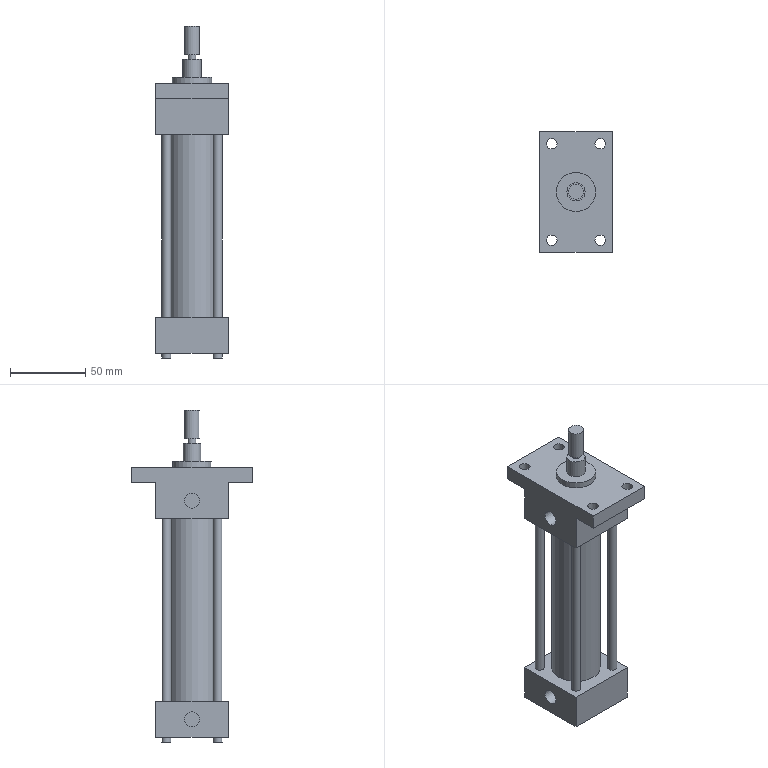Part | NX | features solid 2 | 1 solid | 48 faces | box 48 x 80 x 220 mm | volume 193287 mm3 | plane 28 | cylinder 20 | commonest cylinder face diameters 6 x8 7 x4 10 x3 5 x1 12 x1 26 x1
STEP:
#1=CARTESIAN_POINT('',(-500.,9.,-224.));
#2=VERTEX_POINT('',#1);
#3=CARTESIAN_POINT('',(-516.,9.,-224.));
#4=DIRECTION('',(0.,0.,-1.));
#5=DIRECTION('',(1.,0.,0.));
#6=AXIS2_PLACEMENT_3D('',#3,#4,#5);
#7=CIRCLE('',#6,16.);
#8=EDGE_CURVE('',#2,#2,#7,.T.);
#9=ORIENTED_EDGE('',*,*,#8,.T.);
#10=EDGE_LOOP('',(#9));
#11=FACE_BOUND('',#10,.T.);
#12=CARTESIAN_POINT('',(-500.,9.,-345.));
#13=VERTEX_POINT('',#12);
#14=CARTESIAN_POINT('',(-516.,9.,-345.));
#15=DIRECTION('',(0.,0.,-1.));
#16=DIRECTION('',(1.,0.,0.));
#17=AXIS2_PLACEMENT_3D('',#14,#15,#16);
#18=CIRCLE('',#17,16.);
#19=EDGE_CURVE('',#13,#13,#18,.F.);
#20=ORIENTED_EDGE('',*,*,#19,.T.);
#21=EDGE_LOOP('',(#20));
#22=FACE_BOUND('',#21,.T.);
#23=CARTESIAN_POINT('',(-516.,9.,-369.));
#24=DIRECTION('',(0.,0.,1.));
#25=DIRECTION('',(-1.,0.,0.));
#26=AXIS2_PLACEMENT_3D('',#23,#24,#25);
#27=CYLINDRICAL_SURFACE('',#26,16.);
#28=ADVANCED_FACE('',(#11,#22),#27,.T.);
#29=CARTESIAN_POINT('',(-522.,9.,-174.));
#30=VERTEX_POINT('',#29);
#31=CARTESIAN_POINT('',(-516.,9.,-174.));
#32=DIRECTION('',(0.,0.,1.));
#33=DIRECTION('',(-1.,0.,0.));
#34=AXIS2_PLACEMENT_3D('',#31,#32,#33);
#35=CIRCLE('',#34,6.);
#36=EDGE_CURVE('',#30,#30,#35,.T.);
#37=ORIENTED_EDGE('',*,*,#36,.T.);
#38=EDGE_LOOP('',(#37));
#39=FACE_BOUND('',#38,.T.);
#40=CARTESIAN_POINT('',(-518.5,9.,-174.));
#41=VERTEX_POINT('',#40);
#42=CARTESIAN_POINT('',(-516.,9.,-174.));
#43=DIRECTION('',(0.,0.,1.));
#44=DIRECTION('',(-1.,0.,0.));
#45=AXIS2_PLACEMENT_3D('',#42,#43,#44);
#46=CIRCLE('',#45,2.5);
#47=EDGE_CURVE('',#41,#41,#46,.T.);
#48=ORIENTED_EDGE('',*,*,#47,.F.);
#49=EDGE_LOOP('',(#48));
#50=FACE_BOUND('',#49,.T.);
#51=CARTESIAN_POINT('',(-516.,9.,-174.));
#52=DIRECTION('',(0.,0.,1.));
#53=DIRECTION('',(-1.,0.,0.));
#54=AXIS2_PLACEMENT_3D('',#51,#52,#53);
#55=PLANE('',#54);
#56=ADVANCED_FACE('',(#39,#50),#55,.T.);
#57=CARTESIAN_POINT('',(-529.,9.,-186.));
#58=VERTEX_POINT('',#57);
#59=CARTESIAN_POINT('',(-516.,9.,-186.));
#60=DIRECTION('',(0.,0.,1.));
#61=DIRECTION('',(-1.,0.,0.));
#62=AXIS2_PLACEMENT_3D('',#59,#60,#61);
#63=CIRCLE('',#62,13.);
#64=EDGE_CURVE('',#58,#58,#63,.T.);
#65=ORIENTED_EDGE('',*,*,#64,.T.);
#66=EDGE_LOOP('',(#65));
#67=FACE_BOUND('',#66,.T.);
#68=CARTESIAN_POINT('',(-522.,9.,-186.));
#69=VERTEX_POINT('',#68);
#70=CARTESIAN_POINT('',(-516.,9.,-186.));
#71=DIRECTION('',(0.,0.,1.));
#72=DIRECTION('',(-1.,0.,0.));
#73=AXIS2_PLACEMENT_3D('',#70,#71,#72);
#74=CIRCLE('',#73,6.);
#75=EDGE_CURVE('',#69,#69,#74,.F.);
#76=ORIENTED_EDGE('',*,*,#75,.T.);
#77=EDGE_LOOP('',(#76));
#78=FACE_BOUND('',#77,.T.);
#79=CARTESIAN_POINT('',(-516.,9.,-186.));
#80=DIRECTION('',(0.,0.,1.));
#81=DIRECTION('',(-1.,0.,0.));
#82=AXIS2_PLACEMENT_3D('',#79,#80,#81);
#83=PLANE('',#82);
#84=ADVANCED_FACE('',(#67,#78),#83,.T.);
#85=CARTESIAN_POINT('',(-503.5,41.,-190.));
#86=VERTEX_POINT('',#85);
#87=CARTESIAN_POINT('',(-500.,41.,-190.));
#88=DIRECTION('',(0.,0.,1.));
#89=DIRECTION('',(-1.,0.,0.));
#90=AXIS2_PLACEMENT_3D('',#87,#88,#89);
#91=CIRCLE('',#90,3.5);
#92=EDGE_CURVE('',#86,#86,#91,.T.);
#93=ORIENTED_EDGE('',*,*,#92,.F.);
#94=EDGE_LOOP('',(#93));
#95=FACE_BOUND('',#94,.T.);
#96=CARTESIAN_POINT('',(-535.5,-23.,-190.));
#97=VERTEX_POINT('',#96);
#98=CARTESIAN_POINT('',(-532.,-23.,-190.));
#99=DIRECTION('',(0.,0.,1.));
#100=DIRECTION('',(-1.,0.,0.));
#101=AXIS2_PLACEMENT_3D('',#98,#99,#100);
#102=CIRCLE('',#101,3.5);
#103=EDGE_CURVE('',#97,#97,#102,.T.);
#104=ORIENTED_EDGE('',*,*,#103,.F.);
#105=EDGE_LOOP('',(#104));
#106=FACE_BOUND('',#105,.T.);
#107=CARTESIAN_POINT('',(-492.,-31.,-190.));
#108=VERTEX_POINT('',#107);
#109=CARTESIAN_POINT('',(-540.,-31.,-190.));
#110=VERTEX_POINT('',#109);
#111=CARTESIAN_POINT('',(-492.,-31.,-190.));
#112=DIRECTION('',(-1.,0.,0.));
#113=VECTOR('',#112,1000.);
#114=LINE('',#111,#113);
#115=EDGE_CURVE('',#108,#110,#114,.T.);
#116=ORIENTED_EDGE('',*,*,#115,.F.);
#117=CARTESIAN_POINT('',(-492.,49.,-190.));
#118=VERTEX_POINT('',#117);
#119=CARTESIAN_POINT('',(-492.,-15.,-190.));
#120=DIRECTION('',(0.,-1.,0.));
#121=VECTOR('',#120,1000.);
#122=LINE('',#119,#121);
#123=EDGE_CURVE('',#118,#108,#122,.T.);
#124=ORIENTED_EDGE('',*,*,#123,.F.);
#125=CARTESIAN_POINT('',(-540.,49.,-190.));
#126=VERTEX_POINT('',#125);
#127=CARTESIAN_POINT('',(-492.,49.,-190.));
#128=DIRECTION('',(-1.,0.,0.));
#129=VECTOR('',#128,1000.);
#130=LINE('',#127,#129);
#131=EDGE_CURVE('',#118,#126,#130,.T.);
#132=ORIENTED_EDGE('',*,*,#131,.T.);
#133=CARTESIAN_POINT('',(-540.,49.,-190.));
#134=DIRECTION('',(0.,-1.,0.));
#135=VECTOR('',#134,1000.);
#136=LINE('',#133,#135);
#137=EDGE_CURVE('',#126,#110,#136,.T.);
#138=ORIENTED_EDGE('',*,*,#137,.T.);
#139=EDGE_LOOP('',(#116,#124,#132,#138));
#140=FACE_BOUND('',#139,.T.);
#141=CARTESIAN_POINT('',(-503.5,-23.,-190.));
#142=VERTEX_POINT('',#141);
#143=CARTESIAN_POINT('',(-500.,-23.,-190.));
#144=DIRECTION('',(0.,0.,1.));
#145=DIRECTION('',(-1.,0.,0.));
#146=AXIS2_PLACEMENT_3D('',#143,#144,#145);
#147=CIRCLE('',#146,3.5);
#148=EDGE_CURVE('',#142,#142,#147,.T.);
#149=ORIENTED_EDGE('',*,*,#148,.F.);
#150=EDGE_LOOP('',(#149));
#151=FACE_BOUND('',#150,.T.);
#152=CARTESIAN_POINT('',(-535.5,41.,-190.));
#153=VERTEX_POINT('',#152);
#154=CARTESIAN_POINT('',(-532.,41.,-190.));
#155=DIRECTION('',(0.,0.,1.));
#156=DIRECTION('',(-1.,0.,0.));
#157=AXIS2_PLACEMENT_3D('',#154,#155,#156);
#158=CIRCLE('',#157,3.5);
#159=EDGE_CURVE('',#153,#153,#158,.T.);
#160=ORIENTED_EDGE('',*,*,#159,.F.);
#161=EDGE_LOOP('',(#160));
#162=FACE_BOUND('',#161,.T.);
#163=CARTESIAN_POINT('',(-503.,9.,-190.));
#164=VERTEX_POINT('',#163);
#165=CARTESIAN_POINT('',(-516.,9.,-190.));
#166=DIRECTION('',(0.,0.,-1.));
#167=DIRECTION('',(1.,0.,0.));
#168=AXIS2_PLACEMENT_3D('',#165,#166,#167);
#169=CIRCLE('',#168,13.);
#170=EDGE_CURVE('',#164,#164,#169,.F.);
#171=ORIENTED_EDGE('',*,*,#170,.F.);
#172=EDGE_LOOP('',(#171));
#173=FACE_BOUND('',#172,.T.);
#174=CARTESIAN_POINT('',(-540.,-31.,-190.));
#175=DIRECTION('',(0.,0.,-1.));
#176=DIRECTION('',(1.,0.,0.));
#177=AXIS2_PLACEMENT_3D('',#174,#175,#176);
#178=PLANE('',#177);
#179=ADVANCED_FACE('',(#95,#106,#140,#151,#162,#173),#178,.F.);
#180=CARTESIAN_POINT('',(-540.,33.,-200.));
#181=VERTEX_POINT('',#180);
#182=CARTESIAN_POINT('',(-492.,33.,-200.));
#183=VERTEX_POINT('',#182);
#184=CARTESIAN_POINT('',(-540.,33.,-200.));
#185=DIRECTION('',(1.,0.,0.));
#186=VECTOR('',#185,1000.);
#187=LINE('',#184,#186);
#188=EDGE_CURVE('',#181,#183,#187,.T.);
#189=ORIENTED_EDGE('',*,*,#188,.F.);
#190=CARTESIAN_POINT('',(-540.,49.,-200.));
#191=VERTEX_POINT('',#190);
#192=CARTESIAN_POINT('',(-540.,49.,-200.));
#193=DIRECTION('',(0.,-1.,0.));
#194=VECTOR('',#193,1000.);
#195=LINE('',#192,#194);
#196=EDGE_CURVE('',#191,#181,#195,.T.);
#197=ORIENTED_EDGE('',*,*,#196,.F.);
#198=CARTESIAN_POINT('',(-492.,49.,-200.));
#199=VERTEX_POINT('',#198);
#200=CARTESIAN_POINT('',(-492.,49.,-200.));
#201=DIRECTION('',(-1.,0.,0.));
#202=VECTOR('',#201,1000.);
#203=LINE('',#200,#202);
#204=EDGE_CURVE('',#199,#191,#203,.T.);
#205=ORIENTED_EDGE('',*,*,#204,.F.);
#206=CARTESIAN_POINT('',(-492.,-15.,-200.));
#207=DIRECTION('',(0.,-1.,0.));
#208=VECTOR('',#207,1000.);
#209=LINE('',#206,#208);
#210=EDGE_CURVE('',#199,#183,#209,.T.);
#211=ORIENTED_EDGE('',*,*,#210,.T.);
#212=EDGE_LOOP('',(#189,#197,#205,#211));
#213=FACE_BOUND('',#212,.T.);
#214=CARTESIAN_POINT('',(-503.5,41.,-200.));
#215=VERTEX_POINT('',#214);
#216=CARTESIAN_POINT('',(-500.,41.,-200.));
#217=DIRECTION('',(0.,0.,1.));
#218=DIRECTION('',(-1.,0.,0.));
#219=AXIS2_PLACEMENT_3D('',#216,#217,#218);
#220=CIRCLE('',#219,3.5);
#221=EDGE_CURVE('',#215,#215,#220,.T.);
#222=ORIENTED_EDGE('',*,*,#221,.T.);
#223=EDGE_LOOP('',(#222));
#224=FACE_BOUND('',#223,.T.);
#225=CARTESIAN_POINT('',(-535.5,41.,-200.));
#226=VERTEX_POINT('',#225);
#227=CARTESIAN_POINT('',(-532.,41.,-200.));
#228=DIRECTION('',(0.,0.,1.));
#229=DIRECTION('',(-1.,0.,0.));
#230=AXIS2_PLACEMENT_3D('',#227,#228,#229);
#231=CIRCLE('',#230,3.5);
#232=EDGE_CURVE('',#226,#226,#231,.T.);
#233=ORIENTED_EDGE('',*,*,#232,.T.);
#234=EDGE_LOOP('',(#233));
#235=FACE_BOUND('',#234,.T.);
#236=CARTESIAN_POINT('',(-540.,-31.,-200.));
#237=DIRECTION('',(0.,0.,-1.));
#238=DIRECTION('',(1.,0.,0.));
#239=AXIS2_PLACEMENT_3D('',#236,#237,#238);
#240=PLANE('',#239);
#241=ADVANCED_FACE('',(#213,#224,#235),#240,.T.);
#242=ORIENTED_EDGE('',*,*,#115,.T.);
#243=CARTESIAN_POINT('',(-540.,-31.,-200.));
#244=VERTEX_POINT('',#243);
#245=CARTESIAN_POINT('',(-540.,-31.,-200.));
#246=DIRECTION('',(0.,0.,1.));
#247=VECTOR('',#246,1000.);
#248=LINE('',#245,#247);
#249=EDGE_CURVE('',#244,#110,#248,.T.);
#250=ORIENTED_EDGE('',*,*,#249,.F.);
#251=CARTESIAN_POINT('',(-492.,-31.,-200.));
#252=VERTEX_POINT('',#251);
#253=CARTESIAN_POINT('',(-492.,-31.,-200.));
#254=DIRECTION('',(-1.,0.,0.));
#255=VECTOR('',#254,1000.);
#256=LINE('',#253,#255);
#257=EDGE_CURVE('',#252,#244,#256,.T.);
#258=ORIENTED_EDGE('',*,*,#257,.F.);
#259=CARTESIAN_POINT('',(-492.,-31.,-200.));
#260=DIRECTION('',(0.,0.,1.));
#261=VECTOR('',#260,1000.);
#262=LINE('',#259,#261);
#263=EDGE_CURVE('',#252,#108,#262,.T.);
#264=ORIENTED_EDGE('',*,*,#263,.T.);
#265=EDGE_LOOP('',(#242,#250,#258,#264));
#266=FACE_BOUND('',#265,.T.);
#267=CARTESIAN_POINT('',(-492.,-31.,-200.));
#268=DIRECTION('',(0.,1.,0.));
#269=DIRECTION('',(0.,0.,-1.));
#270=AXIS2_PLACEMENT_3D('',#267,#268,#269);
#271=PLANE('',#270);
#272=ADVANCED_FACE('',(#266),#271,.F.);
#273=CARTESIAN_POINT('',(-540.,14.,-212.));
#274=VERTEX_POINT('',#273);
#275=CARTESIAN_POINT('',(-540.,9.,-212.));
#276=DIRECTION('',(1.,0.,0.));
#277=DIRECTION('',(0.,1.,0.));
#278=AXIS2_PLACEMENT_3D('',#275,#276,#277);
#279=CIRCLE('',#278,5.);
#280=EDGE_CURVE('',#274,#274,#279,.T.);
#281=ORIENTED_EDGE('',*,*,#280,.T.);
#282=EDGE_LOOP('',(#281));
#283=FACE_BOUND('',#282,.T.);
#284=ORIENTED_EDGE('',*,*,#137,.F.);
#285=CARTESIAN_POINT('',(-540.,49.,-200.));
#286=DIRECTION('',(0.,0.,1.));
#287=VECTOR('',#286,1000.);
#288=LINE('',#285,#287);
#289=EDGE_CURVE('',#191,#126,#288,.T.);
#290=ORIENTED_EDGE('',*,*,#289,.F.);
#291=ORIENTED_EDGE('',*,*,#196,.T.);
#292=CARTESIAN_POINT('',(-540.,33.,-224.));
#293=VERTEX_POINT('',#292);
#294=CARTESIAN_POINT('',(-540.,33.,-224.));
#295=DIRECTION('',(0.,0.,1.));
#296=VECTOR('',#295,1000.);
#297=LINE('',#294,#296);
#298=EDGE_CURVE('',#293,#181,#297,.T.);
#299=ORIENTED_EDGE('',*,*,#298,.F.);
#300=CARTESIAN_POINT('',(-540.,-15.,-224.));
#301=VERTEX_POINT('',#300);
#302=CARTESIAN_POINT('',(-540.,-15.,-224.));
#303=DIRECTION('',(0.,1.,0.));
#304=VECTOR('',#303,1000.);
#305=LINE('',#302,#304);
#306=EDGE_CURVE('',#301,#293,#305,.T.);
#307=ORIENTED_EDGE('',*,*,#306,.F.);
#308=CARTESIAN_POINT('',(-540.,-15.,-200.));
#309=VERTEX_POINT('',#308);
#310=CARTESIAN_POINT('',(-540.,-15.,-224.));
#311=DIRECTION('',(0.,0.,1.));
#312=VECTOR('',#311,1000.);
#313=LINE('',#310,#312);
#314=EDGE_CURVE('',#301,#309,#313,.T.);
#315=ORIENTED_EDGE('',*,*,#314,.T.);
#316=CARTESIAN_POINT('',(-540.,49.,-200.));
#317=DIRECTION('',(0.,-1.,0.));
#318=VECTOR('',#317,1000.);
#319=LINE('',#316,#318);
#320=EDGE_CURVE('',#309,#244,#319,.T.);
#321=ORIENTED_EDGE('',*,*,#320,.T.);
#322=ORIENTED_EDGE('',*,*,#249,.T.);
#323=EDGE_LOOP('',(#284,#290,#291,#299,#307,#315,#321,#322));
#324=FACE_BOUND('',#323,.T.);
#325=CARTESIAN_POINT('',(-540.,49.,-200.));
#326=DIRECTION('',(-1.,0.,0.));
#327=DIRECTION('',(0.,-1.,0.));
#328=AXIS2_PLACEMENT_3D('',#325,#326,#327);
#329=PLANE('',#328);
#330=ADVANCED_FACE('',(#283,#324),#329,.T.);
#331=ORIENTED_EDGE('',*,*,#131,.F.);
#332=CARTESIAN_POINT('',(-492.,49.,-200.));
#333=DIRECTION('',(0.,0.,1.));
#334=VECTOR('',#333,1000.);
#335=LINE('',#332,#334);
#336=EDGE_CURVE('',#199,#118,#335,.T.);
#337=ORIENTED_EDGE('',*,*,#336,.F.);
#338=ORIENTED_EDGE('',*,*,#204,.T.);
#339=ORIENTED_EDGE('',*,*,#289,.T.);
#340=EDGE_LOOP('',(#331,#337,#338,#339));
#341=FACE_BOUND('',#340,.T.);
#342=CARTESIAN_POINT('',(-492.,49.,-200.));
#343=DIRECTION('',(0.,1.,0.));
#344=DIRECTION('',(0.,0.,-1.));
#345=AXIS2_PLACEMENT_3D('',#342,#343,#344);
#346=PLANE('',#345);
#347=ADVANCED_FACE('',(#341),#346,.T.);
#348=CARTESIAN_POINT('',(-535.5,-23.,-200.));
#349=VERTEX_POINT('',#348);
#350=CARTESIAN_POINT('',(-532.,-23.,-200.));
#351=DIRECTION('',(0.,0.,1.));
#352=DIRECTION('',(-1.,0.,0.));
#353=AXIS2_PLACEMENT_3D('',#350,#351,#352);
#354=CIRCLE('',#353,3.5);
#355=EDGE_CURVE('',#349,#349,#354,.T.);
#356=ORIENTED_EDGE('',*,*,#355,.F.);
#357=EDGE_LOOP('',(#356));
#358=FACE_BOUND('',#357,.T.);
#359=ORIENTED_EDGE('',*,*,#103,.T.);
#360=EDGE_LOOP('',(#359));
#361=FACE_BOUND('',#360,.T.);
#362=CARTESIAN_POINT('',(-532.,-23.,-200.));
#363=DIRECTION('',(0.,0.,1.));
#364=DIRECTION('',(-1.,0.,0.));
#365=AXIS2_PLACEMENT_3D('',#362,#363,#364);
#366=CYLINDRICAL_SURFACE('',#365,3.5);
#367=ADVANCED_FACE('',(#358,#361),#366,.F.);
#368=ORIENTED_EDGE('',*,*,#123,.T.);
#369=ORIENTED_EDGE('',*,*,#263,.F.);
#370=CARTESIAN_POINT('',(-492.,-15.,-200.));
#371=VERTEX_POINT('',#370);
#372=CARTESIAN_POINT('',(-492.,-15.,-200.));
#373=DIRECTION('',(0.,-1.,0.));
#374=VECTOR('',#373,1000.);
#375=LINE('',#372,#374);
#376=EDGE_CURVE('',#371,#252,#375,.T.);
#377=ORIENTED_EDGE('',*,*,#376,.F.);
#378=CARTESIAN_POINT('',(-492.,-15.,-224.));
#379=VERTEX_POINT('',#378);
#380=CARTESIAN_POINT('',(-492.,-15.,-224.));
#381=DIRECTION('',(0.,0.,1.));
#382=VECTOR('',#381,1000.);
#383=LINE('',#380,#382);
#384=EDGE_CURVE('',#379,#371,#383,.T.);
#385=ORIENTED_EDGE('',*,*,#384,.F.);
#386=CARTESIAN_POINT('',(-492.,33.,-224.));
#387=VERTEX_POINT('',#386);
#388=CARTESIAN_POINT('',(-492.,33.,-224.));
#389=DIRECTION('',(0.,-1.,0.));
#390=VECTOR('',#389,1000.);
#391=LINE('',#388,#390);
#392=EDGE_CURVE('',#387,#379,#391,.T.);
#393=ORIENTED_EDGE('',*,*,#392,.F.);
#394=CARTESIAN_POINT('',(-492.,33.,-224.));
#395=DIRECTION('',(0.,0.,1.));
#396=VECTOR('',#395,1000.);
#397=LINE('',#394,#396);
#398=EDGE_CURVE('',#387,#183,#397,.T.);
#399=ORIENTED_EDGE('',*,*,#398,.T.);
#400=ORIENTED_EDGE('',*,*,#210,.F.);
#401=ORIENTED_EDGE('',*,*,#336,.T.);
#402=EDGE_LOOP('',(#368,#369,#377,#385,#393,#399,#400,#401));
#403=FACE_BOUND('',#402,.T.);
#404=CARTESIAN_POINT('',(-492.,-15.,-200.));
#405=DIRECTION('',(-1.,0.,0.));
#406=DIRECTION('',(0.,0.,-1.));
#407=AXIS2_PLACEMENT_3D('',#404,#405,#406);
#408=PLANE('',#407);
#409=ADVANCED_FACE('',(#403),#408,.F.);
#410=CARTESIAN_POINT('',(-503.5,-23.,-200.));
#411=VERTEX_POINT('',#410);
#412=CARTESIAN_POINT('',(-500.,-23.,-200.));
#413=DIRECTION('',(0.,0.,1.));
#414=DIRECTION('',(-1.,0.,0.));
#415=AXIS2_PLACEMENT_3D('',#412,#413,#414);
#416=CIRCLE('',#415,3.5);
#417=EDGE_CURVE('',#411,#411,#416,.T.);
#418=ORIENTED_EDGE('',*,*,#417,.F.);
#419=EDGE_LOOP('',(#418));
#420=FACE_BOUND('',#419,.T.);
#421=ORIENTED_EDGE('',*,*,#148,.T.);
#422=EDGE_LOOP('',(#421));
#423=FACE_BOUND('',#422,.T.);
#424=CARTESIAN_POINT('',(-500.,-23.,-200.));
#425=DIRECTION('',(0.,0.,1.));
#426=DIRECTION('',(-1.,0.,0.));
#427=AXIS2_PLACEMENT_3D('',#424,#425,#426);
#428=CYLINDRICAL_SURFACE('',#427,3.5);
#429=ADVANCED_FACE('',(#420,#423),#428,.F.);
#430=ORIENTED_EDGE('',*,*,#232,.F.);
#431=EDGE_LOOP('',(#430));
#432=FACE_BOUND('',#431,.T.);
#433=ORIENTED_EDGE('',*,*,#159,.T.);
#434=EDGE_LOOP('',(#433));
#435=FACE_BOUND('',#434,.T.);
#436=CARTESIAN_POINT('',(-532.,41.,-200.));
#437=DIRECTION('',(0.,0.,1.));
#438=DIRECTION('',(-1.,0.,0.));
#439=AXIS2_PLACEMENT_3D('',#436,#437,#438);
#440=CYLINDRICAL_SURFACE('',#439,3.5);
#441=ADVANCED_FACE('',(#432,#435),#440,.F.);
#442=ORIENTED_EDGE('',*,*,#221,.F.);
#443=EDGE_LOOP('',(#442));
#444=FACE_BOUND('',#443,.T.);
#445=ORIENTED_EDGE('',*,*,#92,.T.);
#446=EDGE_LOOP('',(#445));
#447=FACE_BOUND('',#446,.T.);
#448=CARTESIAN_POINT('',(-500.,41.,-200.));
#449=DIRECTION('',(0.,0.,1.));
#450=DIRECTION('',(-1.,0.,0.));
#451=AXIS2_PLACEMENT_3D('',#448,#449,#450);
#452=CYLINDRICAL_SURFACE('',#451,3.5);
#453=ADVANCED_FACE('',(#444,#447),#452,.F.);
#454=CARTESIAN_POINT('',(-492.,-15.,-200.));
#455=DIRECTION('',(-1.,0.,0.));
#456=VECTOR('',#455,1000.);
#457=LINE('',#454,#456);
#458=EDGE_CURVE('',#371,#309,#457,.T.);
#459=ORIENTED_EDGE('',*,*,#458,.F.);
#460=ORIENTED_EDGE('',*,*,#376,.T.);
#461=ORIENTED_EDGE('',*,*,#257,.T.);
#462=ORIENTED_EDGE('',*,*,#320,.F.);
#463=EDGE_LOOP('',(#459,#460,#461,#462));
#464=FACE_BOUND('',#463,.T.);
#465=ORIENTED_EDGE('',*,*,#417,.T.);
#466=EDGE_LOOP('',(#465));
#467=FACE_BOUND('',#466,.T.);
#468=ORIENTED_EDGE('',*,*,#355,.T.);
#469=EDGE_LOOP('',(#468));
#470=FACE_BOUND('',#469,.T.);
#471=CARTESIAN_POINT('',(-540.,-31.,-200.));
#472=DIRECTION('',(0.,0.,-1.));
#473=DIRECTION('',(1.,0.,0.));
#474=AXIS2_PLACEMENT_3D('',#471,#472,#473);
#475=PLANE('',#474);
#476=ADVANCED_FACE('',(#464,#467,#470),#475,.T.);
#477=ORIENTED_EDGE('',*,*,#458,.T.);
#478=ORIENTED_EDGE('',*,*,#314,.F.);
#479=CARTESIAN_POINT('',(-492.,-15.,-224.));
#480=DIRECTION('',(-1.,0.,0.));
#481=VECTOR('',#480,1000.);
#482=LINE('',#479,#481);
#483=EDGE_CURVE('',#379,#301,#482,.T.);
#484=ORIENTED_EDGE('',*,*,#483,.F.);
#485=ORIENTED_EDGE('',*,*,#384,.T.);
#486=EDGE_LOOP('',(#477,#478,#484,#485));
#487=FACE_BOUND('',#486,.T.);
#488=CARTESIAN_POINT('',(-492.,-15.,-224.));
#489=DIRECTION('',(0.,1.,0.));
#490=DIRECTION('',(0.,0.,-1.));
#491=AXIS2_PLACEMENT_3D('',#488,#489,#490);
#492=PLANE('',#491);
#493=ADVANCED_FACE('',(#487),#492,.F.);
#494=ORIENTED_EDGE('',*,*,#188,.T.);
#495=ORIENTED_EDGE('',*,*,#398,.F.);
#496=CARTESIAN_POINT('',(-540.,33.,-224.));
#497=DIRECTION('',(1.,0.,0.));
#498=VECTOR('',#497,1000.);
#499=LINE('',#496,#498);
#500=EDGE_CURVE('',#293,#387,#499,.T.);
#501=ORIENTED_EDGE('',*,*,#500,.F.);
#502=ORIENTED_EDGE('',*,*,#298,.T.);
#503=EDGE_LOOP('',(#494,#495,#501,#502));
#504=FACE_BOUND('',#503,.T.);
#505=CARTESIAN_POINT('',(-540.,33.,-224.));
#506=DIRECTION('',(0.,-1.,0.));
#507=DIRECTION('',(0.,0.,1.));
#508=AXIS2_PLACEMENT_3D('',#505,#506,#507);
#509=PLANE('',#508);
#510=ADVANCED_FACE('',(#504),#509,.F.);
#511=CARTESIAN_POINT('',(-530.,-8.,-224.));
#512=VERTEX_POINT('',#511);
#513=CARTESIAN_POINT('',(-533.,-8.,-224.));
#514=DIRECTION('',(0.,0.,-1.));
#515=DIRECTION('',(1.,0.,0.));
#516=AXIS2_PLACEMENT_3D('',#513,#514,#515);
#517=CIRCLE('',#516,3.);
#518=EDGE_CURVE('',#512,#512,#517,.T.);
#519=ORIENTED_EDGE('',*,*,#518,.F.);
#520=EDGE_LOOP('',(#519));
#521=FACE_BOUND('',#520,.T.);
#522=CARTESIAN_POINT('',(-496.,-8.,-224.));
#523=VERTEX_POINT('',#522);
#524=CARTESIAN_POINT('',(-499.,-8.,-224.));
#525=DIRECTION('',(0.,0.,-1.));
#526=DIRECTION('',(1.,0.,0.));
#527=AXIS2_PLACEMENT_3D('',#524,#525,#526);
#528=CIRCLE('',#527,3.);
#529=EDGE_CURVE('',#523,#523,#528,.T.);
#530=ORIENTED_EDGE('',*,*,#529,.F.);
#531=EDGE_LOOP('',(#530));
#532=FACE_BOUND('',#531,.T.);
#533=CARTESIAN_POINT('',(-496.,26.,-224.));
#534=VERTEX_POINT('',#533);
#535=CARTESIAN_POINT('',(-499.,26.,-224.));
#536=DIRECTION('',(0.,0.,-1.));
#537=DIRECTION('',(1.,0.,0.));
#538=AXIS2_PLACEMENT_3D('',#535,#536,#537);
#539=CIRCLE('',#538,3.);
#540=EDGE_CURVE('',#534,#534,#539,.T.);
#541=ORIENTED_EDGE('',*,*,#540,.F.);
#542=EDGE_LOOP('',(#541));
#543=FACE_BOUND('',#542,.T.);
#544=CARTESIAN_POINT('',(-530.,26.,-224.));
#545=VERTEX_POINT('',#544);
#546=CARTESIAN_POINT('',(-533.,26.,-224.));
#547=DIRECTION('',(0.,0.,-1.));
#548=DIRECTION('',(1.,0.,0.));
#549=AXIS2_PLACEMENT_3D('',#546,#547,#548);
#550=CIRCLE('',#549,3.);
#551=EDGE_CURVE('',#545,#545,#550,.T.);
#552=ORIENTED_EDGE('',*,*,#551,.F.);
#553=EDGE_LOOP('',(#552));
#554=FACE_BOUND('',#553,.T.);
#555=ORIENTED_EDGE('',*,*,#8,.F.);
#556=EDGE_LOOP('',(#555));
#557=FACE_BOUND('',#556,.T.);
#558=ORIENTED_EDGE('',*,*,#392,.T.);
#559=ORIENTED_EDGE('',*,*,#483,.T.);
#560=ORIENTED_EDGE('',*,*,#306,.T.);
#561=ORIENTED_EDGE('',*,*,#500,.T.);
#562=EDGE_LOOP('',(#558,#559,#560,#561));
#563=FACE_BOUND('',#562,.T.);
#564=CARTESIAN_POINT('',(-492.,-15.,-224.));
#565=DIRECTION('',(0.,0.,-1.));
#566=DIRECTION('',(1.,0.,0.));
#567=AXIS2_PLACEMENT_3D('',#564,#565,#566);
#568=PLANE('',#567);
#569=ADVANCED_FACE('',(#521,#532,#543,#554,#557,#563),#568,.T.);
#570=ORIENTED_EDGE('',*,*,#64,.F.);
#571=EDGE_LOOP('',(#570));
#572=FACE_BOUND('',#571,.T.);
#573=ORIENTED_EDGE('',*,*,#170,.T.);
#574=EDGE_LOOP('',(#573));
#575=FACE_BOUND('',#574,.T.);
#576=CARTESIAN_POINT('',(-516.,9.,-186.));
#577=DIRECTION('',(0.,0.,-1.));
#578=DIRECTION('',(1.,0.,0.));
#579=AXIS2_PLACEMENT_3D('',#576,#577,#578);
#580=CYLINDRICAL_SURFACE('',#579,13.);
#581=ADVANCED_FACE('',(#572,#575),#580,.T.);
#582=ORIENTED_EDGE('',*,*,#75,.F.);
#583=EDGE_LOOP('',(#582));
#584=FACE_BOUND('',#583,.T.);
#585=ORIENTED_EDGE('',*,*,#36,.F.);
#586=EDGE_LOOP('',(#585));
#587=FACE_BOUND('',#586,.T.);
#588=CARTESIAN_POINT('',(-516.,9.,-174.));
#589=DIRECTION('',(0.,0.,-1.));
#590=DIRECTION('',(1.,0.,0.));
#591=AXIS2_PLACEMENT_3D('',#588,#589,#590);
#592=CYLINDRICAL_SURFACE('',#591,6.);
#593=ADVANCED_FACE('',(#584,#587),#592,.T.);
#594=CARTESIAN_POINT('',(-492.,33.,-345.));
#595=VERTEX_POINT('',#594);
#596=CARTESIAN_POINT('',(-492.,-15.,-345.));
#597=VERTEX_POINT('',#596);
#598=CARTESIAN_POINT('',(-492.,33.,-345.));
#599=DIRECTION('',(0.,-1.,0.));
#600=VECTOR('',#599,1000.);
#601=LINE('',#598,#600);
#602=EDGE_CURVE('',#595,#597,#601,.T.);
#603=ORIENTED_EDGE('',*,*,#602,.T.);
#604=CARTESIAN_POINT('',(-492.,-15.,-369.));
#605=VERTEX_POINT('',#604);
#606=CARTESIAN_POINT('',(-492.,-15.,-369.));
#607=DIRECTION('',(0.,0.,1.));
#608=VECTOR('',#607,1000.);
#609=LINE('',#606,#608);
#610=EDGE_CURVE('',#605,#597,#609,.T.);
#611=ORIENTED_EDGE('',*,*,#610,.F.);
#612=CARTESIAN_POINT('',(-492.,33.,-369.));
#613=VERTEX_POINT('',#612);
#614=CARTESIAN_POINT('',(-492.,33.,-369.));
#615=DIRECTION('',(0.,-1.,0.));
#616=VECTOR('',#615,1000.);
#617=LINE('',#614,#616);
#618=EDGE_CURVE('',#613,#605,#617,.T.);
#619=ORIENTED_EDGE('',*,*,#618,.F.);
#620=CARTESIAN_POINT('',(-492.,33.,-369.));
#621=DIRECTION('',(0.,0.,1.));
#622=VECTOR('',#621,1000.);
#623=LINE('',#620,#622);
#624=EDGE_CURVE('',#613,#595,#623,.T.);
#625=ORIENTED_EDGE('',*,*,#624,.T.);
#626=EDGE_LOOP('',(#603,#611,#619,#625));
#627=FACE_BOUND('',#626,.T.);
#628=CARTESIAN_POINT('',(-492.,33.,-369.));
#629=DIRECTION('',(-1.,0.,0.));
#630=DIRECTION('',(0.,0.,-1.));
#631=AXIS2_PLACEMENT_3D('',#628,#629,#630);
#632=PLANE('',#631);
#633=ADVANCED_FACE('',(#627),#632,.F.);
#634=CARTESIAN_POINT('',(-540.,-15.,-345.));
#635=VERTEX_POINT('',#634);
#636=CARTESIAN_POINT('',(-492.,-15.,-345.));
#637=DIRECTION('',(-1.,0.,0.));
#638=VECTOR('',#637,1000.);
#639=LINE('',#636,#638);
#640=EDGE_CURVE('',#597,#635,#639,.T.);
#641=ORIENTED_EDGE('',*,*,#640,.T.);
#642=CARTESIAN_POINT('',(-540.,-15.,-369.));
#643=VERTEX_POINT('',#642);
#644=CARTESIAN_POINT('',(-540.,-15.,-369.));
#645=DIRECTION('',(0.,0.,1.));
#646=VECTOR('',#645,1000.);
#647=LINE('',#644,#646);
#648=EDGE_CURVE('',#643,#635,#647,.T.);
#649=ORIENTED_EDGE('',*,*,#648,.F.);
#650=CARTESIAN_POINT('',(-492.,-15.,-369.));
#651=DIRECTION('',(-1.,0.,0.));
#652=VECTOR('',#651,1000.);
#653=LINE('',#650,#652);
#654=EDGE_CURVE('',#605,#643,#653,.T.);
#655=ORIENTED_EDGE('',*,*,#654,.F.);
#656=ORIENTED_EDGE('',*,*,#610,.T.);
#657=EDGE_LOOP('',(#641,#649,#655,#656));
#658=FACE_BOUND('',#657,.T.);
#659=CARTESIAN_POINT('',(-492.,-15.,-369.));
#660=DIRECTION('',(0.,1.,0.));
#661=DIRECTION('',(0.,0.,-1.));
#662=AXIS2_PLACEMENT_3D('',#659,#660,#661);
#663=PLANE('',#662);
#664=ADVANCED_FACE('',(#658),#663,.F.);
#665=CARTESIAN_POINT('',(-540.,14.,-357.));
#666=VERTEX_POINT('',#665);
#667=CARTESIAN_POINT('',(-540.,9.,-357.));
#668=DIRECTION('',(1.,0.,0.));
#669=DIRECTION('',(0.,1.,0.));
#670=AXIS2_PLACEMENT_3D('',#667,#668,#669);
#671=CIRCLE('',#670,5.);
#672=EDGE_CURVE('',#666,#666,#671,.T.);
#673=ORIENTED_EDGE('',*,*,#672,.T.);
#674=EDGE_LOOP('',(#673));
#675=FACE_BOUND('',#674,.T.);
#676=CARTESIAN_POINT('',(-540.,33.,-345.));
#677=VERTEX_POINT('',#676);
#678=CARTESIAN_POINT('',(-540.,-15.,-345.));
#679=DIRECTION('',(0.,1.,0.));
#680=VECTOR('',#679,1000.);
#681=LINE('',#678,#680);
#682=EDGE_CURVE('',#635,#677,#681,.T.);
#683=ORIENTED_EDGE('',*,*,#682,.T.);
#684=CARTESIAN_POINT('',(-540.,33.,-369.));
#685=VERTEX_POINT('',#684);
#686=CARTESIAN_POINT('',(-540.,33.,-369.));
#687=DIRECTION('',(0.,0.,1.));
#688=VECTOR('',#687,1000.);
#689=LINE('',#686,#688);
#690=EDGE_CURVE('',#685,#677,#689,.T.);
#691=ORIENTED_EDGE('',*,*,#690,.F.);
#692=CARTESIAN_POINT('',(-540.,-15.,-369.));
#693=DIRECTION('',(0.,1.,0.));
#694=VECTOR('',#693,1000.);
#695=LINE('',#692,#694);
#696=EDGE_CURVE('',#643,#685,#695,.T.);
#697=ORIENTED_EDGE('',*,*,#696,.F.);
#698=ORIENTED_EDGE('',*,*,#648,.T.);
#699=EDGE_LOOP('',(#683,#691,#697,#698));
#700=FACE_BOUND('',#699,.T.);
#701=CARTESIAN_POINT('',(-540.,-15.,-369.));
#702=DIRECTION('',(1.,0.,0.));
#703=DIRECTION('',(0.,1.,0.));
#704=AXIS2_PLACEMENT_3D('',#701,#702,#703);
#705=PLANE('',#704);
#706=ADVANCED_FACE('',(#675,#700),#705,.F.);
#707=CARTESIAN_POINT('',(-540.,33.,-345.));
#708=DIRECTION('',(1.,0.,0.));
#709=VECTOR('',#708,1000.);
#710=LINE('',#707,#709);
#711=EDGE_CURVE('',#677,#595,#710,.T.);
#712=ORIENTED_EDGE('',*,*,#711,.T.);
#713=ORIENTED_EDGE('',*,*,#624,.F.);
#714=CARTESIAN_POINT('',(-540.,33.,-369.));
#715=DIRECTION('',(1.,0.,0.));
#716=VECTOR('',#715,1000.);
#717=LINE('',#714,#716);
#718=EDGE_CURVE('',#685,#613,#717,.T.);
#719=ORIENTED_EDGE('',*,*,#718,.F.);
#720=ORIENTED_EDGE('',*,*,#690,.T.);
#721=EDGE_LOOP('',(#712,#713,#719,#720));
#722=FACE_BOUND('',#721,.T.);
#723=CARTESIAN_POINT('',(-540.,33.,-369.));
#724=DIRECTION('',(0.,-1.,0.));
#725=DIRECTION('',(0.,0.,1.));
#726=AXIS2_PLACEMENT_3D('',#723,#724,#725);
#727=PLANE('',#726);
#728=ADVANCED_FACE('',(#722),#727,.F.);
#729=CARTESIAN_POINT('',(-530.,-8.,-345.));
#730=VERTEX_POINT('',#729);
#731=CARTESIAN_POINT('',(-533.,-8.,-345.));
#732=DIRECTION('',(0.,0.,-1.));
#733=DIRECTION('',(1.,0.,0.));
#734=AXIS2_PLACEMENT_3D('',#731,#732,#733);
#735=CIRCLE('',#734,3.);
#736=EDGE_CURVE('',#730,#730,#735,.T.);
#737=ORIENTED_EDGE('',*,*,#736,.T.);
#738=EDGE_LOOP('',(#737));
#739=FACE_BOUND('',#738,.T.);
#740=CARTESIAN_POINT('',(-496.,-8.,-345.));
#741=VERTEX_POINT('',#740);
#742=CARTESIAN_POINT('',(-499.,-8.,-345.));
#743=DIRECTION('',(0.,0.,-1.));
#744=DIRECTION('',(1.,0.,0.));
#745=AXIS2_PLACEMENT_3D('',#742,#743,#744);
#746=CIRCLE('',#745,3.);
#747=EDGE_CURVE('',#741,#741,#746,.T.);
#748=ORIENTED_EDGE('',*,*,#747,.T.);
#749=EDGE_LOOP('',(#748));
#750=FACE_BOUND('',#749,.T.);
#751=CARTESIAN_POINT('',(-496.,26.,-345.));
#752=VERTEX_POINT('',#751);
#753=CARTESIAN_POINT('',(-499.,26.,-345.));
#754=DIRECTION('',(0.,0.,-1.));
#755=DIRECTION('',(1.,0.,0.));
#756=AXIS2_PLACEMENT_3D('',#753,#754,#755);
#757=CIRCLE('',#756,3.);
#758=EDGE_CURVE('',#752,#752,#757,.T.);
#759=ORIENTED_EDGE('',*,*,#758,.T.);
#760=EDGE_LOOP('',(#759));
#761=FACE_BOUND('',#760,.T.);
#762=CARTESIAN_POINT('',(-530.,26.,-345.));
#763=VERTEX_POINT('',#762);
#764=CARTESIAN_POINT('',(-533.,26.,-345.));
#765=DIRECTION('',(0.,0.,-1.));
#766=DIRECTION('',(1.,0.,0.));
#767=AXIS2_PLACEMENT_3D('',#764,#765,#766);
#768=CIRCLE('',#767,3.);
#769=EDGE_CURVE('',#763,#763,#768,.T.);
#770=ORIENTED_EDGE('',*,*,#769,.T.);
#771=EDGE_LOOP('',(#770));
#772=FACE_BOUND('',#771,.T.);
#773=ORIENTED_EDGE('',*,*,#19,.F.);
#774=EDGE_LOOP('',(#773));
#775=FACE_BOUND('',#774,.T.);
#776=ORIENTED_EDGE('',*,*,#602,.F.);
#777=ORIENTED_EDGE('',*,*,#711,.F.);
#778=ORIENTED_EDGE('',*,*,#682,.F.);
#779=ORIENTED_EDGE('',*,*,#640,.F.);
#780=EDGE_LOOP('',(#776,#777,#778,#779));
#781=FACE_BOUND('',#780,.T.);
#782=CARTESIAN_POINT('',(-492.,-15.,-345.));
#783=DIRECTION('',(0.,0.,-1.));
#784=DIRECTION('',(1.,0.,0.));
#785=AXIS2_PLACEMENT_3D('',#782,#783,#784);
#786=PLANE('',#785);
#787=ADVANCED_FACE('',(#739,#750,#761,#772,#775,#781),#786,.F.);
#788=CARTESIAN_POINT('',(-536.,-8.,-369.));
#789=VERTEX_POINT('',#788);
#790=CARTESIAN_POINT('',(-533.,-8.,-369.));
#791=DIRECTION('',(0.,0.,1.));
#792=DIRECTION('',(-1.,0.,0.));
#793=AXIS2_PLACEMENT_3D('',#790,#791,#792);
#794=CIRCLE('',#793,3.);
#795=EDGE_CURVE('',#789,#789,#794,.T.);
#796=ORIENTED_EDGE('',*,*,#795,.T.);
#797=EDGE_LOOP('',(#796));
#798=FACE_BOUND('',#797,.T.);
#799=CARTESIAN_POINT('',(-502.,-8.,-369.));
#800=VERTEX_POINT('',#799);
#801=CARTESIAN_POINT('',(-499.,-8.,-369.));
#802=DIRECTION('',(0.,0.,1.));
#803=DIRECTION('',(-1.,0.,0.));
#804=AXIS2_PLACEMENT_3D('',#801,#802,#803);
#805=CIRCLE('',#804,3.);
#806=EDGE_CURVE('',#800,#800,#805,.T.);
#807=ORIENTED_EDGE('',*,*,#806,.T.);
#808=EDGE_LOOP('',(#807));
#809=FACE_BOUND('',#808,.T.);
#810=CARTESIAN_POINT('',(-502.,26.,-369.));
#811=VERTEX_POINT('',#810);
#812=CARTESIAN_POINT('',(-499.,26.,-369.));
#813=DIRECTION('',(0.,0.,1.));
#814=DIRECTION('',(-1.,0.,0.));
#815=AXIS2_PLACEMENT_3D('',#812,#813,#814);
#816=CIRCLE('',#815,3.);
#817=EDGE_CURVE('',#811,#811,#816,.T.);
#818=ORIENTED_EDGE('',*,*,#817,.T.);
#819=EDGE_LOOP('',(#818));
#820=FACE_BOUND('',#819,.T.);
#821=CARTESIAN_POINT('',(-536.,26.,-369.));
#822=VERTEX_POINT('',#821);
#823=CARTESIAN_POINT('',(-533.,26.,-369.));
#824=DIRECTION('',(0.,0.,1.));
#825=DIRECTION('',(-1.,0.,0.));
#826=AXIS2_PLACEMENT_3D('',#823,#824,#825);
#827=CIRCLE('',#826,3.);
#828=EDGE_CURVE('',#822,#822,#827,.T.);
#829=ORIENTED_EDGE('',*,*,#828,.T.);
#830=EDGE_LOOP('',(#829));
#831=FACE_BOUND('',#830,.T.);
#832=ORIENTED_EDGE('',*,*,#618,.T.);
#833=ORIENTED_EDGE('',*,*,#654,.T.);
#834=ORIENTED_EDGE('',*,*,#696,.T.);
#835=ORIENTED_EDGE('',*,*,#718,.T.);
#836=EDGE_LOOP('',(#832,#833,#834,#835));
#837=FACE_BOUND('',#836,.T.);
#838=CARTESIAN_POINT('',(-516.,9.,-369.));
#839=DIRECTION('',(0.,0.,1.));
#840=DIRECTION('',(-1.,0.,0.));
#841=AXIS2_PLACEMENT_3D('',#838,#839,#840);
#842=PLANE('',#841);
#843=ADVANCED_FACE('',(#798,#809,#820,#831,#837),#842,.F.);
#844=CARTESIAN_POINT('',(-536.,26.,-372.));
#845=VERTEX_POINT('',#844);
#846=CARTESIAN_POINT('',(-533.,26.,-372.));
#847=DIRECTION('',(0.,0.,1.));
#848=DIRECTION('',(-1.,0.,0.));
#849=AXIS2_PLACEMENT_3D('',#846,#847,#848);
#850=CIRCLE('',#849,3.);
#851=EDGE_CURVE('',#845,#845,#850,.T.);
#852=ORIENTED_EDGE('',*,*,#851,.F.);
#853=EDGE_LOOP('',(#852));
#854=FACE_BOUND('',#853,.T.);
#855=CARTESIAN_POINT('',(-533.,26.,-372.));
#856=DIRECTION('',(0.,0.,1.));
#857=DIRECTION('',(-1.,0.,0.));
#858=AXIS2_PLACEMENT_3D('',#855,#856,#857);
#859=PLANE('',#858);
#860=ADVANCED_FACE('',(#854),#859,.F.);
#861=ORIENTED_EDGE('',*,*,#851,.T.);
#862=EDGE_LOOP('',(#861));
#863=FACE_BOUND('',#862,.T.);
#864=ORIENTED_EDGE('',*,*,#828,.F.);
#865=EDGE_LOOP('',(#864));
#866=FACE_BOUND('',#865,.T.);
#867=CARTESIAN_POINT('',(-533.,26.,-372.));
#868=DIRECTION('',(0.,0.,1.));
#869=DIRECTION('',(-1.,0.,0.));
#870=AXIS2_PLACEMENT_3D('',#867,#868,#869);
#871=CYLINDRICAL_SURFACE('',#870,3.);
#872=ADVANCED_FACE('',(#863,#866),#871,.T.);
#873=ORIENTED_EDGE('',*,*,#551,.T.);
#874=EDGE_LOOP('',(#873));
#875=FACE_BOUND('',#874,.T.);
#876=ORIENTED_EDGE('',*,*,#769,.F.);
#877=EDGE_LOOP('',(#876));
#878=FACE_BOUND('',#877,.T.);
#879=CARTESIAN_POINT('',(-533.,26.,-372.));
#880=DIRECTION('',(0.,0.,1.));
#881=DIRECTION('',(-1.,0.,0.));
#882=AXIS2_PLACEMENT_3D('',#879,#880,#881);
#883=CYLINDRICAL_SURFACE('',#882,3.);
#884=ADVANCED_FACE('',(#875,#878),#883,.T.);
#885=CARTESIAN_POINT('',(-502.,26.,-372.));
#886=VERTEX_POINT('',#885);
#887=CARTESIAN_POINT('',(-499.,26.,-372.));
#888=DIRECTION('',(0.,0.,1.));
#889=DIRECTION('',(-1.,0.,0.));
#890=AXIS2_PLACEMENT_3D('',#887,#888,#889);
#891=CIRCLE('',#890,3.);
#892=EDGE_CURVE('',#886,#886,#891,.T.);
#893=ORIENTED_EDGE('',*,*,#892,.F.);
#894=EDGE_LOOP('',(#893));
#895=FACE_BOUND('',#894,.T.);
#896=CARTESIAN_POINT('',(-499.,26.,-372.));
#897=DIRECTION('',(0.,0.,1.));
#898=DIRECTION('',(-1.,0.,0.));
#899=AXIS2_PLACEMENT_3D('',#896,#897,#898);
#900=PLANE('',#899);
#901=ADVANCED_FACE('',(#895),#900,.F.);
#902=ORIENTED_EDGE('',*,*,#892,.T.);
#903=EDGE_LOOP('',(#902));
#904=FACE_BOUND('',#903,.T.);
#905=ORIENTED_EDGE('',*,*,#817,.F.);
#906=EDGE_LOOP('',(#905));
#907=FACE_BOUND('',#906,.T.);
#908=CARTESIAN_POINT('',(-499.,26.,-372.));
#909=DIRECTION('',(0.,0.,1.));
#910=DIRECTION('',(-1.,0.,0.));
#911=AXIS2_PLACEMENT_3D('',#908,#909,#910);
#912=CYLINDRICAL_SURFACE('',#911,3.);
#913=ADVANCED_FACE('',(#904,#907),#912,.T.);
#914=ORIENTED_EDGE('',*,*,#540,.T.);
#915=EDGE_LOOP('',(#914));
#916=FACE_BOUND('',#915,.T.);
#917=ORIENTED_EDGE('',*,*,#758,.F.);
#918=EDGE_LOOP('',(#917));
#919=FACE_BOUND('',#918,.T.);
#920=CARTESIAN_POINT('',(-499.,26.,-372.));
#921=DIRECTION('',(0.,0.,1.));
#922=DIRECTION('',(-1.,0.,0.));
#923=AXIS2_PLACEMENT_3D('',#920,#921,#922);
#924=CYLINDRICAL_SURFACE('',#923,3.);
#925=ADVANCED_FACE('',(#916,#919),#924,.T.);
#926=CARTESIAN_POINT('',(-502.,-8.,-372.));
#927=VERTEX_POINT('',#926);
#928=CARTESIAN_POINT('',(-499.,-8.,-372.));
#929=DIRECTION('',(0.,0.,1.));
#930=DIRECTION('',(-1.,0.,0.));
#931=AXIS2_PLACEMENT_3D('',#928,#929,#930);
#932=CIRCLE('',#931,3.);
#933=EDGE_CURVE('',#927,#927,#932,.T.);
#934=ORIENTED_EDGE('',*,*,#933,.F.);
#935=EDGE_LOOP('',(#934));
#936=FACE_BOUND('',#935,.T.);
#937=CARTESIAN_POINT('',(-499.,-8.,-372.));
#938=DIRECTION('',(0.,0.,1.));
#939=DIRECTION('',(-1.,0.,0.));
#940=AXIS2_PLACEMENT_3D('',#937,#938,#939);
#941=PLANE('',#940);
#942=ADVANCED_FACE('',(#936),#941,.F.);
#943=ORIENTED_EDGE('',*,*,#933,.T.);
#944=EDGE_LOOP('',(#943));
#945=FACE_BOUND('',#944,.T.);
#946=ORIENTED_EDGE('',*,*,#806,.F.);
#947=EDGE_LOOP('',(#946));
#948=FACE_BOUND('',#947,.T.);
#949=CARTESIAN_POINT('',(-499.,-8.,-372.));
#950=DIRECTION('',(0.,0.,1.));
#951=DIRECTION('',(-1.,0.,0.));
#952=AXIS2_PLACEMENT_3D('',#949,#950,#951);
#953=CYLINDRICAL_SURFACE('',#952,3.);
#954=ADVANCED_FACE('',(#945,#948),#953,.T.);
#955=ORIENTED_EDGE('',*,*,#529,.T.);
#956=EDGE_LOOP('',(#955));
#957=FACE_BOUND('',#956,.T.);
#958=ORIENTED_EDGE('',*,*,#747,.F.);
#959=EDGE_LOOP('',(#958));
#960=FACE_BOUND('',#959,.T.);
#961=CARTESIAN_POINT('',(-499.,-8.,-372.));
#962=DIRECTION('',(0.,0.,1.));
#963=DIRECTION('',(-1.,0.,0.));
#964=AXIS2_PLACEMENT_3D('',#961,#962,#963);
#965=CYLINDRICAL_SURFACE('',#964,3.);
#966=ADVANCED_FACE('',(#957,#960),#965,.T.);
#967=CARTESIAN_POINT('',(-536.,-8.,-372.));
#968=VERTEX_POINT('',#967);
#969=CARTESIAN_POINT('',(-533.,-8.,-372.));
#970=DIRECTION('',(0.,0.,1.));
#971=DIRECTION('',(-1.,0.,0.));
#972=AXIS2_PLACEMENT_3D('',#969,#970,#971);
#973=CIRCLE('',#972,3.);
#974=EDGE_CURVE('',#968,#968,#973,.T.);
#975=ORIENTED_EDGE('',*,*,#974,.F.);
#976=EDGE_LOOP('',(#975));
#977=FACE_BOUND('',#976,.T.);
#978=CARTESIAN_POINT('',(-533.,-8.,-372.));
#979=DIRECTION('',(0.,0.,1.));
#980=DIRECTION('',(-1.,0.,0.));
#981=AXIS2_PLACEMENT_3D('',#978,#979,#980);
#982=PLANE('',#981);
#983=ADVANCED_FACE('',(#977),#982,.F.);
#984=ORIENTED_EDGE('',*,*,#974,.T.);
#985=EDGE_LOOP('',(#984));
#986=FACE_BOUND('',#985,.T.);
#987=ORIENTED_EDGE('',*,*,#795,.F.);
#988=EDGE_LOOP('',(#987));
#989=FACE_BOUND('',#988,.T.);
#990=CARTESIAN_POINT('',(-533.,-8.,-372.));
#991=DIRECTION('',(0.,0.,1.));
#992=DIRECTION('',(-1.,0.,0.));
#993=AXIS2_PLACEMENT_3D('',#990,#991,#992);
#994=CYLINDRICAL_SURFACE('',#993,3.);
#995=ADVANCED_FACE('',(#986,#989),#994,.T.);
#996=ORIENTED_EDGE('',*,*,#518,.T.);
#997=EDGE_LOOP('',(#996));
#998=FACE_BOUND('',#997,.T.);
#999=ORIENTED_EDGE('',*,*,#736,.F.);
#1000=EDGE_LOOP('',(#999));
#1001=FACE_BOUND('',#1000,.T.);
#1002=CARTESIAN_POINT('',(-533.,-8.,-372.));
#1003=DIRECTION('',(0.,0.,1.));
#1004=DIRECTION('',(-1.,0.,0.));
#1005=AXIS2_PLACEMENT_3D('',#1002,#1003,#1004);
#1006=CYLINDRICAL_SURFACE('',#1005,3.);
#1007=ADVANCED_FACE('',(#998,#1001),#1006,.T.);
#1008=CARTESIAN_POINT('',(-518.5,9.,-171.));
#1009=VERTEX_POINT('',#1008);
#1010=CARTESIAN_POINT('',(-516.,9.,-171.));
#1011=DIRECTION('',(0.,0.,1.));
#1012=DIRECTION('',(-1.,0.,0.));
#1013=AXIS2_PLACEMENT_3D('',#1010,#1011,#1012);
#1014=CIRCLE('',#1013,2.5);
#1015=EDGE_CURVE('',#1009,#1009,#1014,.T.);
#1016=ORIENTED_EDGE('',*,*,#1015,.T.);
#1017=EDGE_LOOP('',(#1016));
#1018=FACE_BOUND('',#1017,.T.);
#1019=CARTESIAN_POINT('',(-521.,9.,-171.));
#1020=VERTEX_POINT('',#1019);
#1021=CARTESIAN_POINT('',(-516.,9.,-171.));
#1022=DIRECTION('',(0.,0.,1.));
#1023=DIRECTION('',(-1.,0.,0.));
#1024=AXIS2_PLACEMENT_3D('',#1021,#1022,#1023);
#1025=CIRCLE('',#1024,5.);
#1026=EDGE_CURVE('',#1020,#1020,#1025,.T.);
#1027=ORIENTED_EDGE('',*,*,#1026,.F.);
#1028=EDGE_LOOP('',(#1027));
#1029=FACE_BOUND('',#1028,.T.);
#1030=CARTESIAN_POINT('',(-516.,9.,-171.));
#1031=DIRECTION('',(0.,0.,1.));
#1032=DIRECTION('',(-1.,0.,0.));
#1033=AXIS2_PLACEMENT_3D('',#1030,#1031,#1032);
#1034=PLANE('',#1033);
#1035=ADVANCED_FACE('',(#1018,#1029),#1034,.F.);
#1036=ORIENTED_EDGE('',*,*,#1015,.F.);
#1037=EDGE_LOOP('',(#1036));
#1038=FACE_BOUND('',#1037,.T.);
#1039=ORIENTED_EDGE('',*,*,#47,.T.);
#1040=EDGE_LOOP('',(#1039));
#1041=FACE_BOUND('',#1040,.T.);
#1042=CARTESIAN_POINT('',(-516.,9.,-172.5));
#1043=DIRECTION('',(0.,0.,1.));
#1044=DIRECTION('',(-1.,0.,0.));
#1045=AXIS2_PLACEMENT_3D('',#1042,#1043,#1044);
#1046=CYLINDRICAL_SURFACE('',#1045,2.5);
#1047=ADVANCED_FACE('',(#1038,#1041),#1046,.T.);
#1048=CARTESIAN_POINT('',(-521.,9.,-152.));
#1049=VERTEX_POINT('',#1048);
#1050=CARTESIAN_POINT('',(-516.,9.,-152.));
#1051=DIRECTION('',(0.,0.,1.));
#1052=DIRECTION('',(-1.,0.,0.));
#1053=AXIS2_PLACEMENT_3D('',#1050,#1051,#1052);
#1054=CIRCLE('',#1053,5.);
#1055=EDGE_CURVE('',#1049,#1049,#1054,.T.);
#1056=ORIENTED_EDGE('',*,*,#1055,.T.);
#1057=EDGE_LOOP('',(#1056));
#1058=FACE_BOUND('',#1057,.T.);
#1059=CARTESIAN_POINT('',(-516.,9.,-152.));
#1060=DIRECTION('',(0.,0.,1.));
#1061=DIRECTION('',(-1.,0.,0.));
#1062=AXIS2_PLACEMENT_3D('',#1059,#1060,#1061);
#1063=PLANE('',#1062);
#1064=ADVANCED_FACE('',(#1058),#1063,.T.);
#1065=ORIENTED_EDGE('',*,*,#1026,.T.);
#1066=EDGE_LOOP('',(#1065));
#1067=FACE_BOUND('',#1066,.T.);
#1068=ORIENTED_EDGE('',*,*,#1055,.F.);
#1069=EDGE_LOOP('',(#1068));
#1070=FACE_BOUND('',#1069,.T.);
#1071=CARTESIAN_POINT('',(-516.,9.,-152.));
#1072=DIRECTION('',(0.,0.,-1.));
#1073=DIRECTION('',(1.,0.,0.));
#1074=AXIS2_PLACEMENT_3D('',#1071,#1072,#1073);
#1075=CYLINDRICAL_SURFACE('',#1074,5.);
#1076=ADVANCED_FACE('',(#1067,#1070),#1075,.T.);
#1077=CARTESIAN_POINT('',(-532.,14.,-212.));
#1078=VERTEX_POINT('',#1077);
#1079=CARTESIAN_POINT('',(-532.,9.,-212.));
#1080=DIRECTION('',(1.,0.,0.));
#1081=DIRECTION('',(0.,1.,0.));
#1082=AXIS2_PLACEMENT_3D('',#1079,#1080,#1081);
#1083=CIRCLE('',#1082,5.);
#1084=EDGE_CURVE('',#1078,#1078,#1083,.T.);
#1085=ORIENTED_EDGE('',*,*,#1084,.F.);
#1086=EDGE_LOOP('',(#1085));
#1087=FACE_BOUND('',#1086,.T.);
#1088=CARTESIAN_POINT('',(-532.,9.,-212.));
#1089=DIRECTION('',(1.,0.,0.));
#1090=DIRECTION('',(0.,1.,0.));
#1091=AXIS2_PLACEMENT_3D('',#1088,#1089,#1090);
#1092=PLANE('',#1091);
#1093=ADVANCED_FACE('',(#1087),#1092,.F.);
#1094=ORIENTED_EDGE('',*,*,#1084,.T.);
#1095=EDGE_LOOP('',(#1094));
#1096=FACE_BOUND('',#1095,.T.);
#1097=ORIENTED_EDGE('',*,*,#280,.F.);
#1098=EDGE_LOOP('',(#1097));
#1099=FACE_BOUND('',#1098,.T.);
#1100=CARTESIAN_POINT('',(-540.,9.,-212.));
#1101=DIRECTION('',(1.,0.,0.));
#1102=DIRECTION('',(0.,1.,0.));
#1103=AXIS2_PLACEMENT_3D('',#1100,#1101,#1102);
#1104=CYLINDRICAL_SURFACE('',#1103,5.);
#1105=ADVANCED_FACE('',(#1096,#1099),#1104,.F.);
#1106=CARTESIAN_POINT('',(-532.,14.,-357.));
#1107=VERTEX_POINT('',#1106);
#1108=CARTESIAN_POINT('',(-532.,9.,-357.));
#1109=DIRECTION('',(1.,0.,0.));
#1110=DIRECTION('',(0.,1.,0.));
#1111=AXIS2_PLACEMENT_3D('',#1108,#1109,#1110);
#1112=CIRCLE('',#1111,5.);
#1113=EDGE_CURVE('',#1107,#1107,#1112,.T.);
#1114=ORIENTED_EDGE('',*,*,#1113,.F.);
#1115=EDGE_LOOP('',(#1114));
#1116=FACE_BOUND('',#1115,.T.);
#1117=CARTESIAN_POINT('',(-532.,9.,-357.));
#1118=DIRECTION('',(1.,0.,0.));
#1119=DIRECTION('',(0.,1.,0.));
#1120=AXIS2_PLACEMENT_3D('',#1117,#1118,#1119);
#1121=PLANE('',#1120);
#1122=ADVANCED_FACE('',(#1116),#1121,.F.);
#1123=ORIENTED_EDGE('',*,*,#1113,.T.);
#1124=EDGE_LOOP('',(#1123));
#1125=FACE_BOUND('',#1124,.T.);
#1126=ORIENTED_EDGE('',*,*,#672,.F.);
#1127=EDGE_LOOP('',(#1126));
#1128=FACE_BOUND('',#1127,.T.);
#1129=CARTESIAN_POINT('',(-540.,9.,-357.));
#1130=DIRECTION('',(1.,0.,0.));
#1131=DIRECTION('',(0.,1.,0.));
#1132=AXIS2_PLACEMENT_3D('',#1129,#1130,#1131);
#1133=CYLINDRICAL_SURFACE('',#1132,5.);
#1134=ADVANCED_FACE('',(#1125,#1128),#1133,.F.);
#1135=CLOSED_SHELL('',(#28,#56,#84,#179,#241,#272,#330,#347,#367,#409,#429,#441,#453,#476,#493,#510,#569,#581,#593,#633,#664,#706,#728,#787,#843,#860,#872,#884,#901,#913,#925,#942,#954,#966,#983,#995,#1007,#1035,#1047,#1064,#1076,#1093,#1105,#1122,#1134));
#1136=CARTESIAN_POINT('',(-529.5,9.,-345.));
#1137=VERTEX_POINT('',#1136);
#1138=CARTESIAN_POINT('',(-516.,9.,-345.));
#1139=DIRECTION('',(0.,0.,1.));
#1140=DIRECTION('',(-1.,0.,0.));
#1141=AXIS2_PLACEMENT_3D('',#1138,#1139,#1140);
#1142=CIRCLE('',#1141,13.5);
#1143=EDGE_CURVE('',#1137,#1137,#1142,.T.);
#1144=ORIENTED_EDGE('',*,*,#1143,.F.);
#1145=EDGE_LOOP('',(#1144));
#1146=FACE_BOUND('',#1145,.T.);
#1147=CARTESIAN_POINT('',(-529.5,9.,-224.));
#1148=VERTEX_POINT('',#1147);
#1149=CARTESIAN_POINT('',(-516.,9.,-224.));
#1150=DIRECTION('',(0.,0.,1.));
#1151=DIRECTION('',(-1.,0.,0.));
#1152=AXIS2_PLACEMENT_3D('',#1149,#1150,#1151);
#1153=CIRCLE('',#1152,13.5);
#1154=EDGE_CURVE('',#1148,#1148,#1153,.T.);
#1155=ORIENTED_EDGE('',*,*,#1154,.T.);
#1156=EDGE_LOOP('',(#1155));
#1157=FACE_BOUND('',#1156,.T.);
#1158=CARTESIAN_POINT('',(-516.,9.,-345.));
#1159=DIRECTION('',(0.,0.,1.));
#1160=DIRECTION('',(-1.,0.,0.));
#1161=AXIS2_PLACEMENT_3D('',#1158,#1159,#1160);
#1162=CYLINDRICAL_SURFACE('',#1161,13.5);
#1163=ADVANCED_FACE('',(#1146,#1157),#1162,.F.);
#1164=ORIENTED_EDGE('',*,*,#1143,.T.);
#1165=EDGE_LOOP('',(#1164));
#1166=FACE_BOUND('',#1165,.T.);
#1167=CARTESIAN_POINT('',(-516.,9.,-345.));
#1168=DIRECTION('',(0.,0.,1.));
#1169=DIRECTION('',(-1.,0.,0.));
#1170=AXIS2_PLACEMENT_3D('',#1167,#1168,#1169);
#1171=PLANE('',#1170);
#1172=ADVANCED_FACE('',(#1166),#1171,.T.);
#1173=ORIENTED_EDGE('',*,*,#1154,.F.);
#1174=EDGE_LOOP('',(#1173));
#1175=FACE_BOUND('',#1174,.T.);
#1176=CARTESIAN_POINT('',(-516.,9.,-224.));
#1177=DIRECTION('',(0.,0.,1.));
#1178=DIRECTION('',(-1.,0.,0.));
#1179=AXIS2_PLACEMENT_3D('',#1176,#1177,#1178);
#1180=PLANE('',#1179);
#1181=ADVANCED_FACE('',(#1175),#1180,.F.);
#1182=CLOSED_SHELL('',(#1163,#1172,#1181));
#1183=ORIENTED_CLOSED_SHELL('',*,#1182,.F.);
#1184=BREP_WITH_VOIDS('',#1135,(#1183));
#1185=(LENGTH_UNIT()NAMED_UNIT(*)SI_UNIT(.MILLI.,.METRE.));
#1186=UNCERTAINTY_MEASURE_WITH_UNIT(LENGTH_MEASURE(0.00001),#1185,'','');
#1187=(NAMED_UNIT(*)PLANE_ANGLE_UNIT()SI_UNIT($,.RADIAN.));
#1188=(NAMED_UNIT(*)SI_UNIT($,.STERADIAN.)SOLID_ANGLE_UNIT());
#1189=(GEOMETRIC_REPRESENTATION_CONTEXT(3)GLOBAL_UNCERTAINTY_ASSIGNED_CONTEXT((#1186))GLOBAL_UNIT_ASSIGNED_CONTEXT((#1185,#1187,#1188))REPRESENTATION_CONTEXT('',''));
#1190=ADVANCED_BREP_SHAPE_REPRESENTATION('',(#1184),#1189);